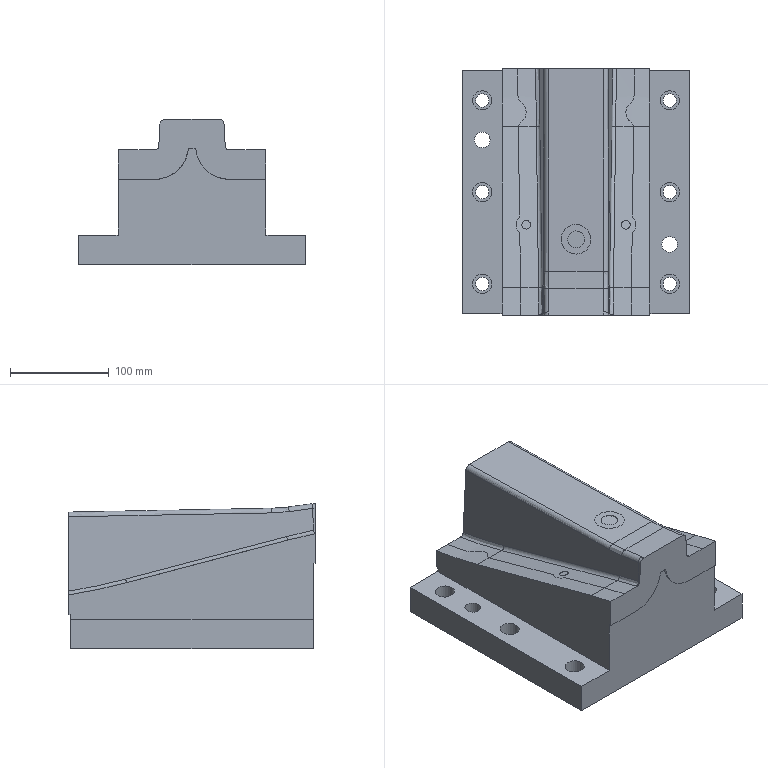Part | NX | features solid 2 | 1 solid | 74 faces | box 230 x 250 x 147.39 mm | volume 4629523 mm3 | spline 41 | plane 18 | cylinder 15 | commonest cylinder face diameters 13.5 x6 19.5 x6 16 x2 17 x1